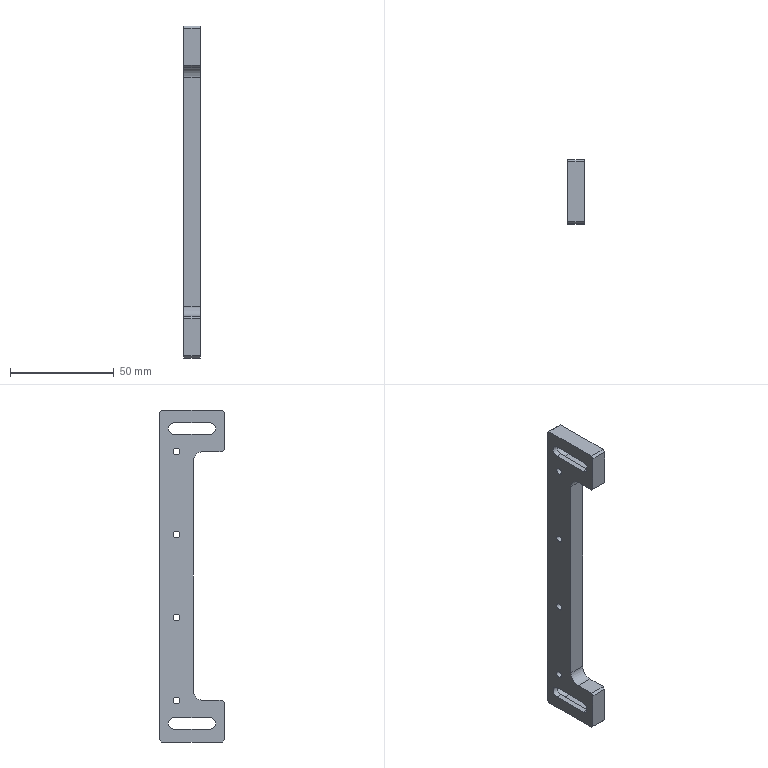Part | SolidWorks | features BaseBody 1 | 1 solid | 44 faces | box 8 x 31 x 160 mm | volume 21339 mm3 | plane 26 | cylinder 18 | commonest cylinder face diameters 3.3 x8 5.5 x4 11 x4 10 x2
STEP:
#1=CARTESIAN_POINT('',(-732.66,-691.086,-336.969));
#2=VERTEX_POINT('',#1);
#3=CARTESIAN_POINT('',(-732.66,-691.086,-333.669));
#4=VERTEX_POINT('',#3);
#5=CARTESIAN_POINT('',(-732.66,-691.086,-335.319));
#6=DIRECTION('',(-1.,0.,0.));
#7=DIRECTION('',(0.,0.,-1.));
#8=AXIS2_PLACEMENT_3D('',#5,#6,#7);
#9=CIRCLE('',#8,1.65);
#10=EDGE_CURVE('',#2,#4,#9,.T.);
#11=ORIENTED_EDGE('',*,*,#10,.T.);
#12=CARTESIAN_POINT('',(-724.66,-691.086,-333.669));
#13=VERTEX_POINT('',#12);
#14=CARTESIAN_POINT('',(-724.66,-691.086,-333.669));
#15=DIRECTION('',(1.,0.,0.));
#16=VECTOR('',#15,1000.);
#17=LINE('',#14,#16);
#18=EDGE_CURVE('',#4,#13,#17,.T.);
#19=ORIENTED_EDGE('',*,*,#18,.T.);
#20=CARTESIAN_POINT('',(-724.66,-691.086,-336.969));
#21=VERTEX_POINT('',#20);
#22=CARTESIAN_POINT('',(-724.66,-691.086,-335.319));
#23=DIRECTION('',(-1.,0.,0.));
#24=DIRECTION('',(0.,0.,-1.));
#25=AXIS2_PLACEMENT_3D('',#22,#23,#24);
#26=CIRCLE('',#25,1.65);
#27=EDGE_CURVE('',#21,#13,#26,.T.);
#28=ORIENTED_EDGE('',*,*,#27,.F.);
#29=CARTESIAN_POINT('',(-724.66,-691.086,-336.969));
#30=DIRECTION('',(1.,0.,0.));
#31=VECTOR('',#30,1000.);
#32=LINE('',#29,#31);
#33=EDGE_CURVE('',#2,#21,#32,.T.);
#34=ORIENTED_EDGE('',*,*,#33,.F.);
#35=EDGE_LOOP('',(#11,#19,#28,#34));
#36=FACE_OUTER_BOUND('',#35,.T.);
#37=CARTESIAN_POINT('',(-724.66,-691.086,-335.319));
#38=DIRECTION('',(1.,0.,0.));
#39=DIRECTION('',(0.,0.,-1.));
#40=AXIS2_PLACEMENT_3D('',#37,#38,#39);
#41=CYLINDRICAL_SURFACE('',#40,1.65);
#42=ADVANCED_FACE('',(#36),#41,.F.);
#43=CARTESIAN_POINT('',(-732.66,-691.086,-376.969));
#44=VERTEX_POINT('',#43);
#45=CARTESIAN_POINT('',(-732.66,-691.086,-373.669));
#46=VERTEX_POINT('',#45);
#47=CARTESIAN_POINT('',(-732.66,-691.086,-375.319));
#48=DIRECTION('',(-1.,0.,0.));
#49=DIRECTION('',(0.,0.,-1.));
#50=AXIS2_PLACEMENT_3D('',#47,#48,#49);
#51=CIRCLE('',#50,1.65);
#52=EDGE_CURVE('',#44,#46,#51,.T.);
#53=ORIENTED_EDGE('',*,*,#52,.T.);
#54=CARTESIAN_POINT('',(-724.66,-691.086,-373.669));
#55=VERTEX_POINT('',#54);
#56=CARTESIAN_POINT('',(-724.66,-691.086,-373.669));
#57=DIRECTION('',(1.,0.,0.));
#58=VECTOR('',#57,1000.);
#59=LINE('',#56,#58);
#60=EDGE_CURVE('',#46,#55,#59,.T.);
#61=ORIENTED_EDGE('',*,*,#60,.T.);
#62=CARTESIAN_POINT('',(-724.66,-691.086,-376.969));
#63=VERTEX_POINT('',#62);
#64=CARTESIAN_POINT('',(-724.66,-691.086,-375.319));
#65=DIRECTION('',(-1.,0.,0.));
#66=DIRECTION('',(0.,0.,-1.));
#67=AXIS2_PLACEMENT_3D('',#64,#65,#66);
#68=CIRCLE('',#67,1.65);
#69=EDGE_CURVE('',#63,#55,#68,.T.);
#70=ORIENTED_EDGE('',*,*,#69,.F.);
#71=CARTESIAN_POINT('',(-724.66,-691.086,-376.969));
#72=DIRECTION('',(1.,0.,0.));
#73=VECTOR('',#72,1000.);
#74=LINE('',#71,#73);
#75=EDGE_CURVE('',#44,#63,#74,.T.);
#76=ORIENTED_EDGE('',*,*,#75,.F.);
#77=EDGE_LOOP('',(#53,#61,#70,#76));
#78=FACE_OUTER_BOUND('',#77,.T.);
#79=CARTESIAN_POINT('',(-724.66,-691.086,-375.319));
#80=DIRECTION('',(1.,0.,0.));
#81=DIRECTION('',(0.,0.,-1.));
#82=AXIS2_PLACEMENT_3D('',#79,#80,#81);
#83=CYLINDRICAL_SURFACE('',#82,1.65);
#84=ADVANCED_FACE('',(#78),#83,.F.);
#85=CARTESIAN_POINT('',(-732.66,-691.086,-416.969));
#86=VERTEX_POINT('',#85);
#87=CARTESIAN_POINT('',(-732.66,-691.086,-413.669));
#88=VERTEX_POINT('',#87);
#89=CARTESIAN_POINT('',(-732.66,-691.086,-415.319));
#90=DIRECTION('',(-1.,0.,0.));
#91=DIRECTION('',(0.,0.,-1.));
#92=AXIS2_PLACEMENT_3D('',#89,#90,#91);
#93=CIRCLE('',#92,1.65);
#94=EDGE_CURVE('',#86,#88,#93,.T.);
#95=ORIENTED_EDGE('',*,*,#94,.T.);
#96=CARTESIAN_POINT('',(-724.66,-691.086,-413.669));
#97=VERTEX_POINT('',#96);
#98=CARTESIAN_POINT('',(-724.66,-691.086,-413.669));
#99=DIRECTION('',(1.,0.,0.));
#100=VECTOR('',#99,1000.);
#101=LINE('',#98,#100);
#102=EDGE_CURVE('',#88,#97,#101,.T.);
#103=ORIENTED_EDGE('',*,*,#102,.T.);
#104=CARTESIAN_POINT('',(-724.66,-691.086,-416.969));
#105=VERTEX_POINT('',#104);
#106=CARTESIAN_POINT('',(-724.66,-691.086,-415.319));
#107=DIRECTION('',(-1.,0.,0.));
#108=DIRECTION('',(0.,0.,-1.));
#109=AXIS2_PLACEMENT_3D('',#106,#107,#108);
#110=CIRCLE('',#109,1.65);
#111=EDGE_CURVE('',#105,#97,#110,.T.);
#112=ORIENTED_EDGE('',*,*,#111,.F.);
#113=CARTESIAN_POINT('',(-724.66,-691.086,-416.969));
#114=DIRECTION('',(1.,0.,0.));
#115=VECTOR('',#114,1000.);
#116=LINE('',#113,#115);
#117=EDGE_CURVE('',#86,#105,#116,.T.);
#118=ORIENTED_EDGE('',*,*,#117,.F.);
#119=EDGE_LOOP('',(#95,#103,#112,#118));
#120=FACE_OUTER_BOUND('',#119,.T.);
#121=CARTESIAN_POINT('',(-724.66,-691.086,-415.319));
#122=DIRECTION('',(1.,0.,0.));
#123=DIRECTION('',(0.,0.,-1.));
#124=AXIS2_PLACEMENT_3D('',#121,#122,#123);
#125=CYLINDRICAL_SURFACE('',#124,1.65);
#126=ADVANCED_FACE('',(#120),#125,.F.);
#127=CARTESIAN_POINT('',(-732.66,-691.086,-456.969));
#128=VERTEX_POINT('',#127);
#129=CARTESIAN_POINT('',(-732.66,-691.086,-453.669));
#130=VERTEX_POINT('',#129);
#131=CARTESIAN_POINT('',(-732.66,-691.086,-455.319));
#132=DIRECTION('',(-1.,0.,0.));
#133=DIRECTION('',(0.,0.,-1.));
#134=AXIS2_PLACEMENT_3D('',#131,#132,#133);
#135=CIRCLE('',#134,1.65);
#136=EDGE_CURVE('',#128,#130,#135,.T.);
#137=ORIENTED_EDGE('',*,*,#136,.T.);
#138=CARTESIAN_POINT('',(-724.66,-691.086,-453.669));
#139=VERTEX_POINT('',#138);
#140=CARTESIAN_POINT('',(-724.66,-691.086,-453.669));
#141=DIRECTION('',(1.,0.,0.));
#142=VECTOR('',#141,1000.);
#143=LINE('',#140,#142);
#144=EDGE_CURVE('',#130,#139,#143,.T.);
#145=ORIENTED_EDGE('',*,*,#144,.T.);
#146=CARTESIAN_POINT('',(-724.66,-691.086,-456.969));
#147=VERTEX_POINT('',#146);
#148=CARTESIAN_POINT('',(-724.66,-691.086,-455.319));
#149=DIRECTION('',(-1.,0.,0.));
#150=DIRECTION('',(0.,0.,-1.));
#151=AXIS2_PLACEMENT_3D('',#148,#149,#150);
#152=CIRCLE('',#151,1.65);
#153=EDGE_CURVE('',#147,#139,#152,.T.);
#154=ORIENTED_EDGE('',*,*,#153,.F.);
#155=CARTESIAN_POINT('',(-724.66,-691.086,-456.969));
#156=DIRECTION('',(1.,0.,0.));
#157=VECTOR('',#156,1000.);
#158=LINE('',#155,#157);
#159=EDGE_CURVE('',#128,#147,#158,.T.);
#160=ORIENTED_EDGE('',*,*,#159,.F.);
#161=EDGE_LOOP('',(#137,#145,#154,#160));
#162=FACE_OUTER_BOUND('',#161,.T.);
#163=CARTESIAN_POINT('',(-724.66,-691.086,-455.319));
#164=DIRECTION('',(1.,0.,0.));
#165=DIRECTION('',(0.,0.,-1.));
#166=AXIS2_PLACEMENT_3D('',#163,#164,#165);
#167=CYLINDRICAL_SURFACE('',#166,1.65);
#168=ADVANCED_FACE('',(#162),#167,.F.);
#169=ORIENTED_EDGE('',*,*,#10,.F.);
#170=CARTESIAN_POINT('',(-732.66,-691.086,-335.319));
#171=DIRECTION('',(-1.,0.,0.));
#172=DIRECTION('',(0.,0.,-1.));
#173=AXIS2_PLACEMENT_3D('',#170,#171,#172);
#174=CIRCLE('',#173,1.65);
#175=EDGE_CURVE('',#4,#2,#174,.T.);
#176=ORIENTED_EDGE('',*,*,#175,.F.);
#177=EDGE_LOOP('',(#169,#176));
#178=FACE_BOUND('',#177,.T.);
#179=ORIENTED_EDGE('',*,*,#52,.F.);
#180=CARTESIAN_POINT('',(-732.66,-691.086,-375.319));
#181=DIRECTION('',(-1.,0.,0.));
#182=DIRECTION('',(0.,0.,-1.));
#183=AXIS2_PLACEMENT_3D('',#180,#181,#182);
#184=CIRCLE('',#183,1.65);
#185=EDGE_CURVE('',#46,#44,#184,.T.);
#186=ORIENTED_EDGE('',*,*,#185,.F.);
#187=EDGE_LOOP('',(#179,#186));
#188=FACE_BOUND('',#187,.T.);
#189=ORIENTED_EDGE('',*,*,#94,.F.);
#190=CARTESIAN_POINT('',(-732.66,-691.086,-415.319));
#191=DIRECTION('',(-1.,0.,0.));
#192=DIRECTION('',(0.,0.,-1.));
#193=AXIS2_PLACEMENT_3D('',#190,#191,#192);
#194=CIRCLE('',#193,1.65);
#195=EDGE_CURVE('',#88,#86,#194,.T.);
#196=ORIENTED_EDGE('',*,*,#195,.F.);
#197=EDGE_LOOP('',(#189,#196));
#198=FACE_BOUND('',#197,.T.);
#199=ORIENTED_EDGE('',*,*,#136,.F.);
#200=CARTESIAN_POINT('',(-732.66,-691.086,-455.319));
#201=DIRECTION('',(-1.,0.,0.));
#202=DIRECTION('',(0.,0.,-1.));
#203=AXIS2_PLACEMENT_3D('',#200,#201,#202);
#204=CIRCLE('',#203,1.65);
#205=EDGE_CURVE('',#130,#128,#204,.T.);
#206=ORIENTED_EDGE('',*,*,#205,.F.);
#207=EDGE_LOOP('',(#199,#206));
#208=FACE_BOUND('',#207,.T.);
#209=CARTESIAN_POINT('',(-732.66,-707.336,-327.069));
#210=VERTEX_POINT('',#209);
#211=CARTESIAN_POINT('',(-732.66,-707.336,-321.569));
#212=VERTEX_POINT('',#211);
#213=CARTESIAN_POINT('',(-732.66,-707.336,-324.319));
#214=DIRECTION('',(-1.,0.,0.));
#215=DIRECTION('',(0.,0.,-1.));
#216=AXIS2_PLACEMENT_3D('',#213,#214,#215);
#217=CIRCLE('',#216,2.75);
#218=EDGE_CURVE('',#210,#212,#217,.T.);
#219=ORIENTED_EDGE('',*,*,#218,.F.);
#220=CARTESIAN_POINT('',(-732.66,-689.836,-327.069));
#221=VERTEX_POINT('',#220);
#222=CARTESIAN_POINT('',(-732.66,-691.086,-327.069));
#223=DIRECTION('',(0.,-1.,0.));
#224=VECTOR('',#223,1000.);
#225=LINE('',#222,#224);
#226=EDGE_CURVE('',#221,#210,#225,.T.);
#227=ORIENTED_EDGE('',*,*,#226,.F.);
#228=CARTESIAN_POINT('',(-732.66,-689.836,-321.569));
#229=VERTEX_POINT('',#228);
#230=CARTESIAN_POINT('',(-732.66,-689.836,-324.319));
#231=DIRECTION('',(-1.,0.,0.));
#232=DIRECTION('',(0.,0.,-1.));
#233=AXIS2_PLACEMENT_3D('',#230,#231,#232);
#234=CIRCLE('',#233,2.75);
#235=EDGE_CURVE('',#229,#221,#234,.T.);
#236=ORIENTED_EDGE('',*,*,#235,.F.);
#237=CARTESIAN_POINT('',(-732.66,-691.086,-321.569));
#238=DIRECTION('',(0.,1.,0.));
#239=VECTOR('',#238,1000.);
#240=LINE('',#237,#239);
#241=EDGE_CURVE('',#212,#229,#240,.T.);
#242=ORIENTED_EDGE('',*,*,#241,.F.);
#243=EDGE_LOOP('',(#219,#227,#236,#242));
#244=FACE_BOUND('',#243,.T.);
#245=CARTESIAN_POINT('',(-732.66,-707.336,-469.069));
#246=VERTEX_POINT('',#245);
#247=CARTESIAN_POINT('',(-732.66,-707.336,-463.569));
#248=VERTEX_POINT('',#247);
#249=CARTESIAN_POINT('',(-732.66,-707.336,-466.319));
#250=DIRECTION('',(-1.,0.,0.));
#251=DIRECTION('',(0.,0.,-1.));
#252=AXIS2_PLACEMENT_3D('',#249,#250,#251);
#253=CIRCLE('',#252,2.75);
#254=EDGE_CURVE('',#246,#248,#253,.T.);
#255=ORIENTED_EDGE('',*,*,#254,.F.);
#256=CARTESIAN_POINT('',(-732.66,-689.836,-469.069));
#257=VERTEX_POINT('',#256);
#258=CARTESIAN_POINT('',(-732.66,-691.086,-469.069));
#259=DIRECTION('',(0.,-1.,0.));
#260=VECTOR('',#259,1000.);
#261=LINE('',#258,#260);
#262=EDGE_CURVE('',#257,#246,#261,.T.);
#263=ORIENTED_EDGE('',*,*,#262,.F.);
#264=CARTESIAN_POINT('',(-732.66,-689.836,-463.569));
#265=VERTEX_POINT('',#264);
#266=CARTESIAN_POINT('',(-732.66,-689.836,-466.319));
#267=DIRECTION('',(-1.,0.,0.));
#268=DIRECTION('',(0.,0.,-1.));
#269=AXIS2_PLACEMENT_3D('',#266,#267,#268);
#270=CIRCLE('',#269,2.75);
#271=EDGE_CURVE('',#265,#257,#270,.T.);
#272=ORIENTED_EDGE('',*,*,#271,.F.);
#273=CARTESIAN_POINT('',(-732.66,-691.086,-463.569));
#274=DIRECTION('',(0.,1.,0.));
#275=VECTOR('',#274,1000.);
#276=LINE('',#273,#275);
#277=EDGE_CURVE('',#248,#265,#276,.T.);
#278=ORIENTED_EDGE('',*,*,#277,.F.);
#279=EDGE_LOOP('',(#255,#263,#272,#278));
#280=FACE_BOUND('',#279,.T.);
#281=CARTESIAN_POINT('',(-732.66,-713.086,-335.319));
#282=VERTEX_POINT('',#281);
#283=CARTESIAN_POINT('',(-732.66,-704.086,-335.319));
#284=VERTEX_POINT('',#283);
#285=CARTESIAN_POINT('',(-732.66,-691.086,-335.319));
#286=DIRECTION('',(0.,1.,0.));
#287=VECTOR('',#286,1000.);
#288=LINE('',#285,#287);
#289=EDGE_CURVE('',#282,#284,#288,.T.);
#290=ORIENTED_EDGE('',*,*,#289,.F.);
#291=CARTESIAN_POINT('',(-732.66,-714.086,-334.319));
#292=VERTEX_POINT('',#291);
#293=CARTESIAN_POINT('',(-732.66,-714.086,-334.319));
#294=DIRECTION('',(0.,-0.7071,0.7071));
#295=VECTOR('',#294,1000.);
#296=LINE('',#293,#295);
#297=EDGE_CURVE('',#282,#292,#296,.T.);
#298=ORIENTED_EDGE('',*,*,#297,.T.);
#299=CARTESIAN_POINT('',(-732.66,-714.086,-316.319));
#300=VERTEX_POINT('',#299);
#301=CARTESIAN_POINT('',(-732.66,-714.086,-395.319));
#302=DIRECTION('',(0.,0.,-1.));
#303=VECTOR('',#302,1000.);
#304=LINE('',#301,#303);
#305=EDGE_CURVE('',#300,#292,#304,.T.);
#306=ORIENTED_EDGE('',*,*,#305,.F.);
#307=CARTESIAN_POINT('',(-732.66,-713.086,-315.319));
#308=VERTEX_POINT('',#307);
#309=CARTESIAN_POINT('',(-732.66,-713.086,-315.319));
#310=DIRECTION('',(0.,-0.7071,-0.7071));
#311=VECTOR('',#310,1000.);
#312=LINE('',#309,#311);
#313=EDGE_CURVE('',#308,#300,#312,.T.);
#314=ORIENTED_EDGE('',*,*,#313,.F.);
#315=CARTESIAN_POINT('',(-732.66,-684.086,-315.319));
#316=VERTEX_POINT('',#315);
#317=CARTESIAN_POINT('',(-732.66,-691.086,-315.319));
#318=DIRECTION('',(0.,-1.,0.));
#319=VECTOR('',#318,1000.);
#320=LINE('',#317,#319);
#321=EDGE_CURVE('',#316,#308,#320,.T.);
#322=ORIENTED_EDGE('',*,*,#321,.F.);
#323=CARTESIAN_POINT('',(-732.66,-683.086,-316.319));
#324=VERTEX_POINT('',#323);
#325=CARTESIAN_POINT('',(-732.66,-684.086,-315.319));
#326=DIRECTION('',(0.,0.7071,-0.7071));
#327=VECTOR('',#326,1000.);
#328=LINE('',#325,#327);
#329=EDGE_CURVE('',#316,#324,#328,.T.);
#330=ORIENTED_EDGE('',*,*,#329,.T.);
#331=CARTESIAN_POINT('',(-732.66,-683.086,-474.319));
#332=VERTEX_POINT('',#331);
#333=CARTESIAN_POINT('',(-732.66,-683.086,-395.319));
#334=DIRECTION('',(0.,0.,1.));
#335=VECTOR('',#334,1000.);
#336=LINE('',#333,#335);
#337=EDGE_CURVE('',#332,#324,#336,.T.);
#338=ORIENTED_EDGE('',*,*,#337,.F.);
#339=CARTESIAN_POINT('',(-732.66,-684.086,-475.319));
#340=VERTEX_POINT('',#339);
#341=CARTESIAN_POINT('',(-732.66,-683.086,-474.319));
#342=DIRECTION('',(0.,-0.7071,-0.7071));
#343=VECTOR('',#342,1000.);
#344=LINE('',#341,#343);
#345=EDGE_CURVE('',#332,#340,#344,.T.);
#346=ORIENTED_EDGE('',*,*,#345,.T.);
#347=CARTESIAN_POINT('',(-732.66,-713.086,-475.319));
#348=VERTEX_POINT('',#347);
#349=CARTESIAN_POINT('',(-732.66,-691.086,-475.319));
#350=DIRECTION('',(0.,1.,0.));
#351=VECTOR('',#350,1000.);
#352=LINE('',#349,#351);
#353=EDGE_CURVE('',#348,#340,#352,.T.);
#354=ORIENTED_EDGE('',*,*,#353,.F.);
#355=CARTESIAN_POINT('',(-732.66,-714.086,-474.319));
#356=VERTEX_POINT('',#355);
#357=CARTESIAN_POINT('',(-732.66,-714.086,-474.319));
#358=DIRECTION('',(0.,0.7071,-0.7071));
#359=VECTOR('',#358,1000.);
#360=LINE('',#357,#359);
#361=EDGE_CURVE('',#356,#348,#360,.T.);
#362=ORIENTED_EDGE('',*,*,#361,.F.);
#363=CARTESIAN_POINT('',(-732.66,-714.086,-456.319));
#364=VERTEX_POINT('',#363);
#365=CARTESIAN_POINT('',(-732.66,-714.086,-395.319));
#366=DIRECTION('',(0.,0.,-1.));
#367=VECTOR('',#366,1000.);
#368=LINE('',#365,#367);
#369=EDGE_CURVE('',#364,#356,#368,.T.);
#370=ORIENTED_EDGE('',*,*,#369,.F.);
#371=CARTESIAN_POINT('',(-732.66,-713.086,-455.319));
#372=VERTEX_POINT('',#371);
#373=CARTESIAN_POINT('',(-732.66,-713.086,-455.319));
#374=DIRECTION('',(0.,0.7071,0.7071));
#375=VECTOR('',#374,1000.);
#376=LINE('',#373,#375);
#377=EDGE_CURVE('',#364,#372,#376,.T.);
#378=ORIENTED_EDGE('',*,*,#377,.T.);
#379=CARTESIAN_POINT('',(-732.66,-704.086,-455.319));
#380=VERTEX_POINT('',#379);
#381=CARTESIAN_POINT('',(-732.66,-691.086,-455.319));
#382=DIRECTION('',(0.,-1.,0.));
#383=VECTOR('',#382,1000.);
#384=LINE('',#381,#383);
#385=EDGE_CURVE('',#380,#372,#384,.T.);
#386=ORIENTED_EDGE('',*,*,#385,.F.);
#387=CARTESIAN_POINT('',(-732.66,-699.086,-450.319));
#388=VERTEX_POINT('',#387);
#389=CARTESIAN_POINT('',(-732.66,-704.086,-450.319));
#390=DIRECTION('',(-1.,0.,0.));
#391=DIRECTION('',(0.,0.,-1.));
#392=AXIS2_PLACEMENT_3D('',#389,#390,#391);
#393=CIRCLE('',#392,5.);
#394=EDGE_CURVE('',#388,#380,#393,.T.);
#395=ORIENTED_EDGE('',*,*,#394,.F.);
#396=CARTESIAN_POINT('',(-732.66,-699.086,-340.319));
#397=VERTEX_POINT('',#396);
#398=CARTESIAN_POINT('',(-732.66,-699.086,-395.319));
#399=DIRECTION('',(0.,0.,-1.));
#400=VECTOR('',#399,1000.);
#401=LINE('',#398,#400);
#402=EDGE_CURVE('',#397,#388,#401,.T.);
#403=ORIENTED_EDGE('',*,*,#402,.F.);
#404=CARTESIAN_POINT('',(-732.66,-704.086,-340.319));
#405=DIRECTION('',(-1.,0.,0.));
#406=DIRECTION('',(0.,0.,-1.));
#407=AXIS2_PLACEMENT_3D('',#404,#405,#406);
#408=CIRCLE('',#407,5.);
#409=EDGE_CURVE('',#284,#397,#408,.T.);
#410=ORIENTED_EDGE('',*,*,#409,.F.);
#411=EDGE_LOOP('',(#290,#298,#306,#314,#322,#330,#338,#346,#354,#362,#370,#378,#386,#395,#403,#410));
#412=FACE_OUTER_BOUND('',#411,.T.);
#413=CARTESIAN_POINT('',(-732.66,-691.086,-395.319));
#414=DIRECTION('',(1.,0.,0.));
#415=DIRECTION('',(0.,0.,-1.));
#416=AXIS2_PLACEMENT_3D('',#413,#414,#415);
#417=PLANE('',#416);
#418=ADVANCED_FACE('',(#178,#188,#198,#208,#244,#280,#412),#417,.F.);
#419=ORIENTED_EDGE('',*,*,#18,.F.);
#420=ORIENTED_EDGE('',*,*,#175,.T.);
#421=ORIENTED_EDGE('',*,*,#33,.T.);
#422=CARTESIAN_POINT('',(-724.66,-691.086,-335.319));
#423=DIRECTION('',(-1.,0.,0.));
#424=DIRECTION('',(0.,0.,-1.));
#425=AXIS2_PLACEMENT_3D('',#422,#423,#424);
#426=CIRCLE('',#425,1.65);
#427=EDGE_CURVE('',#13,#21,#426,.T.);
#428=ORIENTED_EDGE('',*,*,#427,.F.);
#429=EDGE_LOOP('',(#419,#420,#421,#428));
#430=FACE_OUTER_BOUND('',#429,.T.);
#431=CARTESIAN_POINT('',(-724.66,-691.086,-335.319));
#432=DIRECTION('',(1.,0.,0.));
#433=DIRECTION('',(0.,0.,-1.));
#434=AXIS2_PLACEMENT_3D('',#431,#432,#433);
#435=CYLINDRICAL_SURFACE('',#434,1.65);
#436=ADVANCED_FACE('',(#430),#435,.F.);
#437=ORIENTED_EDGE('',*,*,#60,.F.);
#438=ORIENTED_EDGE('',*,*,#185,.T.);
#439=ORIENTED_EDGE('',*,*,#75,.T.);
#440=CARTESIAN_POINT('',(-724.66,-691.086,-375.319));
#441=DIRECTION('',(-1.,0.,0.));
#442=DIRECTION('',(0.,0.,-1.));
#443=AXIS2_PLACEMENT_3D('',#440,#441,#442);
#444=CIRCLE('',#443,1.65);
#445=EDGE_CURVE('',#55,#63,#444,.T.);
#446=ORIENTED_EDGE('',*,*,#445,.F.);
#447=EDGE_LOOP('',(#437,#438,#439,#446));
#448=FACE_OUTER_BOUND('',#447,.T.);
#449=CARTESIAN_POINT('',(-724.66,-691.086,-375.319));
#450=DIRECTION('',(1.,0.,0.));
#451=DIRECTION('',(0.,0.,-1.));
#452=AXIS2_PLACEMENT_3D('',#449,#450,#451);
#453=CYLINDRICAL_SURFACE('',#452,1.65);
#454=ADVANCED_FACE('',(#448),#453,.F.);
#455=ORIENTED_EDGE('',*,*,#102,.F.);
#456=ORIENTED_EDGE('',*,*,#195,.T.);
#457=ORIENTED_EDGE('',*,*,#117,.T.);
#458=CARTESIAN_POINT('',(-724.66,-691.086,-415.319));
#459=DIRECTION('',(-1.,0.,0.));
#460=DIRECTION('',(0.,0.,-1.));
#461=AXIS2_PLACEMENT_3D('',#458,#459,#460);
#462=CIRCLE('',#461,1.65);
#463=EDGE_CURVE('',#97,#105,#462,.T.);
#464=ORIENTED_EDGE('',*,*,#463,.F.);
#465=EDGE_LOOP('',(#455,#456,#457,#464));
#466=FACE_OUTER_BOUND('',#465,.T.);
#467=CARTESIAN_POINT('',(-724.66,-691.086,-415.319));
#468=DIRECTION('',(1.,0.,0.));
#469=DIRECTION('',(0.,0.,-1.));
#470=AXIS2_PLACEMENT_3D('',#467,#468,#469);
#471=CYLINDRICAL_SURFACE('',#470,1.65);
#472=ADVANCED_FACE('',(#466),#471,.F.);
#473=ORIENTED_EDGE('',*,*,#144,.F.);
#474=ORIENTED_EDGE('',*,*,#205,.T.);
#475=ORIENTED_EDGE('',*,*,#159,.T.);
#476=CARTESIAN_POINT('',(-724.66,-691.086,-455.319));
#477=DIRECTION('',(-1.,0.,0.));
#478=DIRECTION('',(0.,0.,-1.));
#479=AXIS2_PLACEMENT_3D('',#476,#477,#478);
#480=CIRCLE('',#479,1.65);
#481=EDGE_CURVE('',#139,#147,#480,.T.);
#482=ORIENTED_EDGE('',*,*,#481,.F.);
#483=EDGE_LOOP('',(#473,#474,#475,#482));
#484=FACE_OUTER_BOUND('',#483,.T.);
#485=CARTESIAN_POINT('',(-724.66,-691.086,-455.319));
#486=DIRECTION('',(1.,0.,0.));
#487=DIRECTION('',(0.,0.,-1.));
#488=AXIS2_PLACEMENT_3D('',#485,#486,#487);
#489=CYLINDRICAL_SURFACE('',#488,1.65);
#490=ADVANCED_FACE('',(#484),#489,.F.);
#491=CARTESIAN_POINT('',(-730.06,-707.336,-321.569));
#492=VERTEX_POINT('',#491);
#493=CARTESIAN_POINT('',(-724.66,-707.336,-321.569));
#494=DIRECTION('',(1.,0.,0.));
#495=VECTOR('',#494,1000.);
#496=LINE('',#493,#495);
#497=EDGE_CURVE('',#212,#492,#496,.T.);
#498=ORIENTED_EDGE('',*,*,#497,.F.);
#499=ORIENTED_EDGE('',*,*,#241,.T.);
#500=CARTESIAN_POINT('',(-730.06,-689.836,-321.569));
#501=VERTEX_POINT('',#500);
#502=CARTESIAN_POINT('',(-724.66,-689.836,-321.569));
#503=DIRECTION('',(-1.,0.,0.));
#504=VECTOR('',#503,1000.);
#505=LINE('',#502,#504);
#506=EDGE_CURVE('',#501,#229,#505,.T.);
#507=ORIENTED_EDGE('',*,*,#506,.F.);
#508=CARTESIAN_POINT('',(-730.06,-707.336,-321.569));
#509=DIRECTION('',(0.,1.,0.));
#510=VECTOR('',#509,1000.);
#511=LINE('',#508,#510);
#512=EDGE_CURVE('',#492,#501,#511,.T.);
#513=ORIENTED_EDGE('',*,*,#512,.F.);
#514=EDGE_LOOP('',(#498,#499,#507,#513));
#515=FACE_OUTER_BOUND('',#514,.T.);
#516=CARTESIAN_POINT('',(-724.66,-707.336,-321.569));
#517=DIRECTION('',(0.,0.,1.));
#518=DIRECTION('',(1.,0.,0.));
#519=AXIS2_PLACEMENT_3D('',#516,#517,#518);
#520=PLANE('',#519);
#521=ADVANCED_FACE('',(#515),#520,.F.);
#522=CARTESIAN_POINT('',(-730.06,-707.336,-327.069));
#523=VERTEX_POINT('',#522);
#524=CARTESIAN_POINT('',(-724.66,-707.336,-327.069));
#525=DIRECTION('',(1.,0.,0.));
#526=VECTOR('',#525,1000.);
#527=LINE('',#524,#526);
#528=EDGE_CURVE('',#210,#523,#527,.T.);
#529=ORIENTED_EDGE('',*,*,#528,.F.);
#530=ORIENTED_EDGE('',*,*,#218,.T.);
#531=ORIENTED_EDGE('',*,*,#497,.T.);
#532=CARTESIAN_POINT('',(-730.06,-707.336,-324.319));
#533=DIRECTION('',(-1.,0.,0.));
#534=DIRECTION('',(0.,0.,-1.));
#535=AXIS2_PLACEMENT_3D('',#532,#533,#534);
#536=CIRCLE('',#535,2.75);
#537=EDGE_CURVE('',#523,#492,#536,.T.);
#538=ORIENTED_EDGE('',*,*,#537,.F.);
#539=EDGE_LOOP('',(#529,#530,#531,#538));
#540=FACE_OUTER_BOUND('',#539,.T.);
#541=CARTESIAN_POINT('',(-724.66,-707.336,-324.319));
#542=DIRECTION('',(1.,0.,0.));
#543=DIRECTION('',(0.,0.,-1.));
#544=AXIS2_PLACEMENT_3D('',#541,#542,#543);
#545=CYLINDRICAL_SURFACE('',#544,2.75);
#546=ADVANCED_FACE('',(#540),#545,.F.);
#547=CARTESIAN_POINT('',(-730.06,-689.836,-327.069));
#548=VERTEX_POINT('',#547);
#549=CARTESIAN_POINT('',(-732.66,-689.836,-327.069));
#550=DIRECTION('',(1.,0.,0.));
#551=VECTOR('',#550,1000.);
#552=LINE('',#549,#551);
#553=EDGE_CURVE('',#221,#548,#552,.T.);
#554=ORIENTED_EDGE('',*,*,#553,.F.);
#555=ORIENTED_EDGE('',*,*,#226,.T.);
#556=ORIENTED_EDGE('',*,*,#528,.T.);
#557=CARTESIAN_POINT('',(-730.06,-707.336,-327.069));
#558=DIRECTION('',(0.,-1.,0.));
#559=VECTOR('',#558,1000.);
#560=LINE('',#557,#559);
#561=EDGE_CURVE('',#548,#523,#560,.T.);
#562=ORIENTED_EDGE('',*,*,#561,.F.);
#563=EDGE_LOOP('',(#554,#555,#556,#562));
#564=FACE_OUTER_BOUND('',#563,.T.);
#565=CARTESIAN_POINT('',(-732.66,-707.336,-327.069));
#566=DIRECTION('',(0.,0.,-1.));
#567=DIRECTION('',(0.,1.,0.));
#568=AXIS2_PLACEMENT_3D('',#565,#566,#567);
#569=PLANE('',#568);
#570=ADVANCED_FACE('',(#564),#569,.F.);
#571=ORIENTED_EDGE('',*,*,#506,.T.);
#572=ORIENTED_EDGE('',*,*,#235,.T.);
#573=ORIENTED_EDGE('',*,*,#553,.T.);
#574=CARTESIAN_POINT('',(-730.06,-689.836,-324.319));
#575=DIRECTION('',(-1.,0.,0.));
#576=DIRECTION('',(0.,0.,-1.));
#577=AXIS2_PLACEMENT_3D('',#574,#575,#576);
#578=CIRCLE('',#577,2.75);
#579=EDGE_CURVE('',#501,#548,#578,.T.);
#580=ORIENTED_EDGE('',*,*,#579,.F.);
#581=EDGE_LOOP('',(#571,#572,#573,#580));
#582=FACE_OUTER_BOUND('',#581,.T.);
#583=CARTESIAN_POINT('',(-724.66,-689.836,-324.319));
#584=DIRECTION('',(1.,0.,0.));
#585=DIRECTION('',(0.,0.,-1.));
#586=AXIS2_PLACEMENT_3D('',#583,#584,#585);
#587=CYLINDRICAL_SURFACE('',#586,2.75);
#588=ADVANCED_FACE('',(#582),#587,.F.);
#589=CARTESIAN_POINT('',(-730.06,-707.336,-463.569));
#590=VERTEX_POINT('',#589);
#591=CARTESIAN_POINT('',(-724.66,-707.336,-463.569));
#592=DIRECTION('',(1.,0.,0.));
#593=VECTOR('',#592,1000.);
#594=LINE('',#591,#593);
#595=EDGE_CURVE('',#248,#590,#594,.T.);
#596=ORIENTED_EDGE('',*,*,#595,.F.);
#597=ORIENTED_EDGE('',*,*,#277,.T.);
#598=CARTESIAN_POINT('',(-730.06,-689.836,-463.569));
#599=VERTEX_POINT('',#598);
#600=CARTESIAN_POINT('',(-724.66,-689.836,-463.569));
#601=DIRECTION('',(-1.,0.,0.));
#602=VECTOR('',#601,1000.);
#603=LINE('',#600,#602);
#604=EDGE_CURVE('',#599,#265,#603,.T.);
#605=ORIENTED_EDGE('',*,*,#604,.F.);
#606=CARTESIAN_POINT('',(-730.06,-707.336,-463.569));
#607=DIRECTION('',(0.,1.,0.));
#608=VECTOR('',#607,1000.);
#609=LINE('',#606,#608);
#610=EDGE_CURVE('',#590,#599,#609,.T.);
#611=ORIENTED_EDGE('',*,*,#610,.F.);
#612=EDGE_LOOP('',(#596,#597,#605,#611));
#613=FACE_OUTER_BOUND('',#612,.T.);
#614=CARTESIAN_POINT('',(-724.66,-707.336,-463.569));
#615=DIRECTION('',(0.,0.,1.));
#616=DIRECTION('',(1.,0.,0.));
#617=AXIS2_PLACEMENT_3D('',#614,#615,#616);
#618=PLANE('',#617);
#619=ADVANCED_FACE('',(#613),#618,.F.);
#620=CARTESIAN_POINT('',(-730.06,-707.336,-469.069));
#621=VERTEX_POINT('',#620);
#622=CARTESIAN_POINT('',(-724.66,-707.336,-469.069));
#623=DIRECTION('',(1.,0.,0.));
#624=VECTOR('',#623,1000.);
#625=LINE('',#622,#624);
#626=EDGE_CURVE('',#246,#621,#625,.T.);
#627=ORIENTED_EDGE('',*,*,#626,.F.);
#628=ORIENTED_EDGE('',*,*,#254,.T.);
#629=ORIENTED_EDGE('',*,*,#595,.T.);
#630=CARTESIAN_POINT('',(-730.06,-707.336,-466.319));
#631=DIRECTION('',(-1.,0.,0.));
#632=DIRECTION('',(0.,0.,-1.));
#633=AXIS2_PLACEMENT_3D('',#630,#631,#632);
#634=CIRCLE('',#633,2.75);
#635=EDGE_CURVE('',#621,#590,#634,.T.);
#636=ORIENTED_EDGE('',*,*,#635,.F.);
#637=EDGE_LOOP('',(#627,#628,#629,#636));
#638=FACE_OUTER_BOUND('',#637,.T.);
#639=CARTESIAN_POINT('',(-724.66,-707.336,-466.319));
#640=DIRECTION('',(1.,0.,0.));
#641=DIRECTION('',(0.,0.,-1.));
#642=AXIS2_PLACEMENT_3D('',#639,#640,#641);
#643=CYLINDRICAL_SURFACE('',#642,2.75);
#644=ADVANCED_FACE('',(#638),#643,.F.);
#645=CARTESIAN_POINT('',(-730.06,-689.836,-469.069));
#646=VERTEX_POINT('',#645);
#647=CARTESIAN_POINT('',(-732.66,-689.836,-469.069));
#648=DIRECTION('',(1.,0.,0.));
#649=VECTOR('',#648,1000.);
#650=LINE('',#647,#649);
#651=EDGE_CURVE('',#257,#646,#650,.T.);
#652=ORIENTED_EDGE('',*,*,#651,.F.);
#653=ORIENTED_EDGE('',*,*,#262,.T.);
#654=ORIENTED_EDGE('',*,*,#626,.T.);
#655=CARTESIAN_POINT('',(-730.06,-707.336,-469.069));
#656=DIRECTION('',(0.,-1.,0.));
#657=VECTOR('',#656,1000.);
#658=LINE('',#655,#657);
#659=EDGE_CURVE('',#646,#621,#658,.T.);
#660=ORIENTED_EDGE('',*,*,#659,.F.);
#661=EDGE_LOOP('',(#652,#653,#654,#660));
#662=FACE_OUTER_BOUND('',#661,.T.);
#663=CARTESIAN_POINT('',(-732.66,-707.336,-469.069));
#664=DIRECTION('',(0.,0.,-1.));
#665=DIRECTION('',(0.,1.,0.));
#666=AXIS2_PLACEMENT_3D('',#663,#664,#665);
#667=PLANE('',#666);
#668=ADVANCED_FACE('',(#662),#667,.F.);
#669=ORIENTED_EDGE('',*,*,#604,.T.);
#670=ORIENTED_EDGE('',*,*,#271,.T.);
#671=ORIENTED_EDGE('',*,*,#651,.T.);
#672=CARTESIAN_POINT('',(-730.06,-689.836,-466.319));
#673=DIRECTION('',(-1.,0.,0.));
#674=DIRECTION('',(0.,0.,-1.));
#675=AXIS2_PLACEMENT_3D('',#672,#673,#674);
#676=CIRCLE('',#675,2.75);
#677=EDGE_CURVE('',#599,#646,#676,.T.);
#678=ORIENTED_EDGE('',*,*,#677,.F.);
#679=EDGE_LOOP('',(#669,#670,#671,#678));
#680=FACE_OUTER_BOUND('',#679,.T.);
#681=CARTESIAN_POINT('',(-724.66,-689.836,-466.319));
#682=DIRECTION('',(1.,0.,0.));
#683=DIRECTION('',(0.,0.,-1.));
#684=AXIS2_PLACEMENT_3D('',#681,#682,#683);
#685=CYLINDRICAL_SURFACE('',#684,2.75);
#686=ADVANCED_FACE('',(#680),#685,.F.);
#687=CARTESIAN_POINT('',(-724.66,-704.086,-335.319));
#688=VERTEX_POINT('',#687);
#689=CARTESIAN_POINT('',(-724.66,-699.086,-340.319));
#690=VERTEX_POINT('',#689);
#691=CARTESIAN_POINT('',(-724.66,-704.086,-340.319));
#692=DIRECTION('',(-1.,0.,0.));
#693=DIRECTION('',(0.,0.,-1.));
#694=AXIS2_PLACEMENT_3D('',#691,#692,#693);
#695=CIRCLE('',#694,5.);
#696=EDGE_CURVE('',#688,#690,#695,.T.);
#697=ORIENTED_EDGE('',*,*,#696,.F.);
#698=CARTESIAN_POINT('',(-732.66,-704.086,-335.319));
#699=DIRECTION('',(1.,0.,0.));
#700=VECTOR('',#699,1000.);
#701=LINE('',#698,#700);
#702=EDGE_CURVE('',#284,#688,#701,.T.);
#703=ORIENTED_EDGE('',*,*,#702,.F.);
#704=ORIENTED_EDGE('',*,*,#409,.T.);
#705=CARTESIAN_POINT('',(-732.66,-699.086,-340.319));
#706=DIRECTION('',(-1.,0.,0.));
#707=VECTOR('',#706,1000.);
#708=LINE('',#705,#707);
#709=EDGE_CURVE('',#690,#397,#708,.T.);
#710=ORIENTED_EDGE('',*,*,#709,.F.);
#711=EDGE_LOOP('',(#697,#703,#704,#710));
#712=FACE_OUTER_BOUND('',#711,.T.);
#713=CARTESIAN_POINT('',(-732.66,-704.086,-340.319));
#714=DIRECTION('',(1.,0.,0.));
#715=DIRECTION('',(0.,0.,-1.));
#716=AXIS2_PLACEMENT_3D('',#713,#714,#715);
#717=CYLINDRICAL_SURFACE('',#716,5.);
#718=ADVANCED_FACE('',(#712),#717,.F.);
#719=CARTESIAN_POINT('',(-724.66,-713.086,-335.319));
#720=VERTEX_POINT('',#719);
#721=CARTESIAN_POINT('',(-724.66,-699.086,-335.319));
#722=DIRECTION('',(0.,-1.,0.));
#723=VECTOR('',#722,1000.);
#724=LINE('',#721,#723);
#725=EDGE_CURVE('',#688,#720,#724,.T.);
#726=ORIENTED_EDGE('',*,*,#725,.T.);
#727=CARTESIAN_POINT('',(-732.66,-713.086,-335.319));
#728=DIRECTION('',(-1.,0.,0.));
#729=VECTOR('',#728,1000.);
#730=LINE('',#727,#729);
#731=EDGE_CURVE('',#720,#282,#730,.T.);
#732=ORIENTED_EDGE('',*,*,#731,.T.);
#733=ORIENTED_EDGE('',*,*,#289,.T.);
#734=ORIENTED_EDGE('',*,*,#702,.T.);
#735=EDGE_LOOP('',(#726,#732,#733,#734));
#736=FACE_OUTER_BOUND('',#735,.T.);
#737=CARTESIAN_POINT('',(-732.66,-699.086,-335.319));
#738=DIRECTION('',(0.,0.,-1.));
#739=DIRECTION('',(-1.,0.,0.));
#740=AXIS2_PLACEMENT_3D('',#737,#738,#739);
#741=PLANE('',#740);
#742=ADVANCED_FACE('',(#736),#741,.T.);
#743=ORIENTED_EDGE('',*,*,#305,.T.);
#744=CARTESIAN_POINT('',(-724.66,-714.086,-334.319));
#745=VERTEX_POINT('',#744);
#746=CARTESIAN_POINT('',(-732.66,-714.086,-334.319));
#747=DIRECTION('',(1.,0.,0.));
#748=VECTOR('',#747,1000.);
#749=LINE('',#746,#748);
#750=EDGE_CURVE('',#292,#745,#749,.T.);
#751=ORIENTED_EDGE('',*,*,#750,.T.);
#752=CARTESIAN_POINT('',(-724.66,-714.086,-316.319));
#753=VERTEX_POINT('',#752);
#754=CARTESIAN_POINT('',(-724.66,-714.086,-315.319));
#755=DIRECTION('',(0.,0.,1.));
#756=VECTOR('',#755,1000.);
#757=LINE('',#754,#756);
#758=EDGE_CURVE('',#745,#753,#757,.T.);
#759=ORIENTED_EDGE('',*,*,#758,.T.);
#760=CARTESIAN_POINT('',(-732.66,-714.086,-316.319));
#761=DIRECTION('',(-1.,0.,0.));
#762=VECTOR('',#761,1000.);
#763=LINE('',#760,#762);
#764=EDGE_CURVE('',#753,#300,#763,.T.);
#765=ORIENTED_EDGE('',*,*,#764,.T.);
#766=EDGE_LOOP('',(#743,#751,#759,#765));
#767=FACE_OUTER_BOUND('',#766,.T.);
#768=CARTESIAN_POINT('',(-732.66,-714.086,-315.319));
#769=DIRECTION('',(0.,-1.,0.));
#770=DIRECTION('',(0.,0.,-1.));
#771=AXIS2_PLACEMENT_3D('',#768,#769,#770);
#772=PLANE('',#771);
#773=ADVANCED_FACE('',(#767),#772,.T.);
#774=CARTESIAN_POINT('',(-724.66,-684.086,-315.319));
#775=VERTEX_POINT('',#774);
#776=CARTESIAN_POINT('',(-724.66,-713.086,-315.319));
#777=VERTEX_POINT('',#776);
#778=CARTESIAN_POINT('',(-724.66,-683.086,-315.319));
#779=DIRECTION('',(0.,-1.,0.));
#780=VECTOR('',#779,1000.);
#781=LINE('',#778,#780);
#782=EDGE_CURVE('',#775,#777,#781,.T.);
#783=ORIENTED_EDGE('',*,*,#782,.F.);
#784=CARTESIAN_POINT('',(-724.66,-684.086,-315.319));
#785=DIRECTION('',(1.,0.,0.));
#786=VECTOR('',#785,1000.);
#787=LINE('',#784,#786);
#788=EDGE_CURVE('',#316,#775,#787,.T.);
#789=ORIENTED_EDGE('',*,*,#788,.F.);
#790=ORIENTED_EDGE('',*,*,#321,.T.);
#791=CARTESIAN_POINT('',(-724.66,-713.086,-315.319));
#792=DIRECTION('',(-1.,0.,0.));
#793=VECTOR('',#792,1000.);
#794=LINE('',#791,#793);
#795=EDGE_CURVE('',#777,#308,#794,.T.);
#796=ORIENTED_EDGE('',*,*,#795,.F.);
#797=EDGE_LOOP('',(#783,#789,#790,#796));
#798=FACE_OUTER_BOUND('',#797,.T.);
#799=CARTESIAN_POINT('',(-724.66,-683.086,-315.319));
#800=DIRECTION('',(0.,0.,-1.));
#801=DIRECTION('',(-1.,0.,0.));
#802=AXIS2_PLACEMENT_3D('',#799,#800,#801);
#803=PLANE('',#802);
#804=ADVANCED_FACE('',(#798),#803,.F.);
#805=ORIENTED_EDGE('',*,*,#337,.T.);
#806=CARTESIAN_POINT('',(-724.66,-683.086,-316.319));
#807=VERTEX_POINT('',#806);
#808=CARTESIAN_POINT('',(-724.66,-683.086,-316.319));
#809=DIRECTION('',(-1.,0.,0.));
#810=VECTOR('',#809,1000.);
#811=LINE('',#808,#810);
#812=EDGE_CURVE('',#807,#324,#811,.T.);
#813=ORIENTED_EDGE('',*,*,#812,.F.);
#814=CARTESIAN_POINT('',(-724.66,-683.086,-474.319));
#815=VERTEX_POINT('',#814);
#816=CARTESIAN_POINT('',(-724.66,-683.086,-315.319));
#817=DIRECTION('',(0.,0.,1.));
#818=VECTOR('',#817,1000.);
#819=LINE('',#816,#818);
#820=EDGE_CURVE('',#815,#807,#819,.T.);
#821=ORIENTED_EDGE('',*,*,#820,.F.);
#822=CARTESIAN_POINT('',(-724.66,-683.086,-474.319));
#823=DIRECTION('',(1.,0.,0.));
#824=VECTOR('',#823,1000.);
#825=LINE('',#822,#824);
#826=EDGE_CURVE('',#332,#815,#825,.T.);
#827=ORIENTED_EDGE('',*,*,#826,.F.);
#828=EDGE_LOOP('',(#805,#813,#821,#827));
#829=FACE_OUTER_BOUND('',#828,.T.);
#830=CARTESIAN_POINT('',(-724.66,-683.086,-315.319));
#831=DIRECTION('',(0.,-1.,0.));
#832=DIRECTION('',(1.,0.,0.));
#833=AXIS2_PLACEMENT_3D('',#830,#831,#832);
#834=PLANE('',#833);
#835=ADVANCED_FACE('',(#829),#834,.F.);
#836=ORIENTED_EDGE('',*,*,#353,.T.);
#837=CARTESIAN_POINT('',(-724.66,-684.086,-475.319));
#838=VERTEX_POINT('',#837);
#839=CARTESIAN_POINT('',(-724.66,-684.086,-475.319));
#840=DIRECTION('',(-1.,0.,0.));
#841=VECTOR('',#840,1000.);
#842=LINE('',#839,#841);
#843=EDGE_CURVE('',#838,#340,#842,.T.);
#844=ORIENTED_EDGE('',*,*,#843,.F.);
#845=CARTESIAN_POINT('',(-724.66,-713.086,-475.319));
#846=VERTEX_POINT('',#845);
#847=CARTESIAN_POINT('',(-724.66,-683.086,-475.319));
#848=DIRECTION('',(0.,1.,0.));
#849=VECTOR('',#848,1000.);
#850=LINE('',#847,#849);
#851=EDGE_CURVE('',#846,#838,#850,.T.);
#852=ORIENTED_EDGE('',*,*,#851,.F.);
#853=CARTESIAN_POINT('',(-724.66,-713.086,-475.319));
#854=DIRECTION('',(1.,0.,0.));
#855=VECTOR('',#854,1000.);
#856=LINE('',#853,#855);
#857=EDGE_CURVE('',#348,#846,#856,.T.);
#858=ORIENTED_EDGE('',*,*,#857,.F.);
#859=EDGE_LOOP('',(#836,#844,#852,#858));
#860=FACE_OUTER_BOUND('',#859,.T.);
#861=CARTESIAN_POINT('',(-724.66,-683.086,-475.319));
#862=DIRECTION('',(0.,0.,1.));
#863=DIRECTION('',(1.,0.,0.));
#864=AXIS2_PLACEMENT_3D('',#861,#862,#863);
#865=PLANE('',#864);
#866=ADVANCED_FACE('',(#860),#865,.F.);
#867=CARTESIAN_POINT('',(-724.66,-714.086,-474.319));
#868=VERTEX_POINT('',#867);
#869=CARTESIAN_POINT('',(-724.66,-714.086,-456.319));
#870=VERTEX_POINT('',#869);
#871=CARTESIAN_POINT('',(-724.66,-714.086,-475.319));
#872=DIRECTION('',(0.,0.,1.));
#873=VECTOR('',#872,1000.);
#874=LINE('',#871,#873);
#875=EDGE_CURVE('',#868,#870,#874,.T.);
#876=ORIENTED_EDGE('',*,*,#875,.T.);
#877=CARTESIAN_POINT('',(-732.66,-714.086,-456.319));
#878=DIRECTION('',(-1.,0.,0.));
#879=VECTOR('',#878,1000.);
#880=LINE('',#877,#879);
#881=EDGE_CURVE('',#870,#364,#880,.T.);
#882=ORIENTED_EDGE('',*,*,#881,.T.);
#883=ORIENTED_EDGE('',*,*,#369,.T.);
#884=CARTESIAN_POINT('',(-732.66,-714.086,-474.319));
#885=DIRECTION('',(1.,0.,0.));
#886=VECTOR('',#885,1000.);
#887=LINE('',#884,#886);
#888=EDGE_CURVE('',#356,#868,#887,.T.);
#889=ORIENTED_EDGE('',*,*,#888,.T.);
#890=EDGE_LOOP('',(#876,#882,#883,#889));
#891=FACE_OUTER_BOUND('',#890,.T.);
#892=CARTESIAN_POINT('',(-732.66,-714.086,-475.319));
#893=DIRECTION('',(0.,-1.,0.));
#894=DIRECTION('',(0.,0.,-1.));
#895=AXIS2_PLACEMENT_3D('',#892,#893,#894);
#896=PLANE('',#895);
#897=ADVANCED_FACE('',(#891),#896,.T.);
#898=ORIENTED_EDGE('',*,*,#385,.T.);
#899=CARTESIAN_POINT('',(-724.66,-713.086,-455.319));
#900=VERTEX_POINT('',#899);
#901=CARTESIAN_POINT('',(-732.66,-713.086,-455.319));
#902=DIRECTION('',(1.,0.,0.));
#903=VECTOR('',#902,1000.);
#904=LINE('',#901,#903);
#905=EDGE_CURVE('',#372,#900,#904,.T.);
#906=ORIENTED_EDGE('',*,*,#905,.T.);
#907=CARTESIAN_POINT('',(-724.66,-704.086,-455.319));
#908=VERTEX_POINT('',#907);
#909=CARTESIAN_POINT('',(-724.66,-699.086,-455.319));
#910=DIRECTION('',(0.,1.,0.));
#911=VECTOR('',#910,1000.);
#912=LINE('',#909,#911);
#913=EDGE_CURVE('',#900,#908,#912,.T.);
#914=ORIENTED_EDGE('',*,*,#913,.T.);
#915=CARTESIAN_POINT('',(-732.66,-704.086,-455.319));
#916=DIRECTION('',(-1.,0.,0.));
#917=VECTOR('',#916,1000.);
#918=LINE('',#915,#917);
#919=EDGE_CURVE('',#908,#380,#918,.T.);
#920=ORIENTED_EDGE('',*,*,#919,.T.);
#921=EDGE_LOOP('',(#898,#906,#914,#920));
#922=FACE_OUTER_BOUND('',#921,.T.);
#923=CARTESIAN_POINT('',(-732.66,-699.086,-455.319));
#924=DIRECTION('',(0.,0.,1.));
#925=DIRECTION('',(1.,0.,0.));
#926=AXIS2_PLACEMENT_3D('',#923,#924,#925);
#927=PLANE('',#926);
#928=ADVANCED_FACE('',(#922),#927,.T.);
#929=CARTESIAN_POINT('',(-724.66,-699.086,-450.319));
#930=VERTEX_POINT('',#929);
#931=CARTESIAN_POINT('',(-724.66,-704.086,-450.319));
#932=DIRECTION('',(-1.,0.,0.));
#933=DIRECTION('',(0.,0.,-1.));
#934=AXIS2_PLACEMENT_3D('',#931,#932,#933);
#935=CIRCLE('',#934,5.);
#936=EDGE_CURVE('',#930,#908,#935,.T.);
#937=ORIENTED_EDGE('',*,*,#936,.F.);
#938=CARTESIAN_POINT('',(-724.66,-699.086,-450.319));
#939=DIRECTION('',(1.,0.,0.));
#940=VECTOR('',#939,1000.);
#941=LINE('',#938,#940);
#942=EDGE_CURVE('',#388,#930,#941,.T.);
#943=ORIENTED_EDGE('',*,*,#942,.F.);
#944=ORIENTED_EDGE('',*,*,#394,.T.);
#945=ORIENTED_EDGE('',*,*,#919,.F.);
#946=EDGE_LOOP('',(#937,#943,#944,#945));
#947=FACE_OUTER_BOUND('',#946,.T.);
#948=CARTESIAN_POINT('',(-724.66,-704.086,-450.319));
#949=DIRECTION('',(1.,0.,0.));
#950=DIRECTION('',(0.,0.,-1.));
#951=AXIS2_PLACEMENT_3D('',#948,#949,#950);
#952=CYLINDRICAL_SURFACE('',#951,5.);
#953=ADVANCED_FACE('',(#947),#952,.F.);
#954=CARTESIAN_POINT('',(-724.66,-699.086,-315.319));
#955=DIRECTION('',(0.,0.,-1.));
#956=VECTOR('',#955,1000.);
#957=LINE('',#954,#956);
#958=EDGE_CURVE('',#690,#930,#957,.T.);
#959=ORIENTED_EDGE('',*,*,#958,.F.);
#960=ORIENTED_EDGE('',*,*,#709,.T.);
#961=ORIENTED_EDGE('',*,*,#402,.T.);
#962=ORIENTED_EDGE('',*,*,#942,.T.);
#963=EDGE_LOOP('',(#959,#960,#961,#962));
#964=FACE_OUTER_BOUND('',#963,.T.);
#965=CARTESIAN_POINT('',(-724.66,-699.086,-315.319));
#966=DIRECTION('',(0.,1.,0.));
#967=DIRECTION('',(0.,0.,1.));
#968=AXIS2_PLACEMENT_3D('',#965,#966,#967);
#969=PLANE('',#968);
#970=ADVANCED_FACE('',(#964),#969,.F.);
#971=ORIENTED_EDGE('',*,*,#27,.T.);
#972=ORIENTED_EDGE('',*,*,#427,.T.);
#973=EDGE_LOOP('',(#971,#972));
#974=FACE_BOUND('',#973,.T.);
#975=ORIENTED_EDGE('',*,*,#69,.T.);
#976=ORIENTED_EDGE('',*,*,#445,.T.);
#977=EDGE_LOOP('',(#975,#976));
#978=FACE_BOUND('',#977,.T.);
#979=ORIENTED_EDGE('',*,*,#111,.T.);
#980=ORIENTED_EDGE('',*,*,#463,.T.);
#981=EDGE_LOOP('',(#979,#980));
#982=FACE_BOUND('',#981,.T.);
#983=ORIENTED_EDGE('',*,*,#153,.T.);
#984=ORIENTED_EDGE('',*,*,#481,.T.);
#985=EDGE_LOOP('',(#983,#984));
#986=FACE_BOUND('',#985,.T.);
#987=CARTESIAN_POINT('',(-724.66,-689.836,-318.819));
#988=VERTEX_POINT('',#987);
#989=CARTESIAN_POINT('',(-724.66,-689.836,-329.819));
#990=VERTEX_POINT('',#989);
#991=CARTESIAN_POINT('',(-724.66,-689.836,-324.319));
#992=DIRECTION('',(-1.,0.,0.));
#993=DIRECTION('',(0.,0.,-1.));
#994=AXIS2_PLACEMENT_3D('',#991,#992,#993);
#995=CIRCLE('',#994,5.5);
#996=EDGE_CURVE('',#988,#990,#995,.T.);
#997=ORIENTED_EDGE('',*,*,#996,.T.);
#998=CARTESIAN_POINT('',(-724.66,-707.336,-329.819));
#999=VERTEX_POINT('',#998);
#1000=CARTESIAN_POINT('',(-724.66,-691.086,-329.819));
#1001=DIRECTION('',(0.,-1.,0.));
#1002=VECTOR('',#1001,1000.);
#1003=LINE('',#1000,#1002);
#1004=EDGE_CURVE('',#990,#999,#1003,.T.);
#1005=ORIENTED_EDGE('',*,*,#1004,.T.);
#1006=CARTESIAN_POINT('',(-724.66,-707.336,-318.819));
#1007=VERTEX_POINT('',#1006);
#1008=CARTESIAN_POINT('',(-724.66,-707.336,-324.319));
#1009=DIRECTION('',(-1.,0.,0.));
#1010=DIRECTION('',(0.,0.,-1.));
#1011=AXIS2_PLACEMENT_3D('',#1008,#1009,#1010);
#1012=CIRCLE('',#1011,5.5);
#1013=EDGE_CURVE('',#999,#1007,#1012,.T.);
#1014=ORIENTED_EDGE('',*,*,#1013,.T.);
#1015=CARTESIAN_POINT('',(-724.66,-691.086,-318.819));
#1016=DIRECTION('',(0.,1.,0.));
#1017=VECTOR('',#1016,1000.);
#1018=LINE('',#1015,#1017);
#1019=EDGE_CURVE('',#1007,#988,#1018,.T.);
#1020=ORIENTED_EDGE('',*,*,#1019,.T.);
#1021=EDGE_LOOP('',(#997,#1005,#1014,#1020));
#1022=FACE_BOUND('',#1021,.T.);
#1023=CARTESIAN_POINT('',(-724.66,-689.836,-460.819));
#1024=VERTEX_POINT('',#1023);
#1025=CARTESIAN_POINT('',(-724.66,-689.836,-471.819));
#1026=VERTEX_POINT('',#1025);
#1027=CARTESIAN_POINT('',(-724.66,-689.836,-466.319));
#1028=DIRECTION('',(-1.,0.,0.));
#1029=DIRECTION('',(0.,0.,-1.));
#1030=AXIS2_PLACEMENT_3D('',#1027,#1028,#1029);
#1031=CIRCLE('',#1030,5.5);
#1032=EDGE_CURVE('',#1024,#1026,#1031,.T.);
#1033=ORIENTED_EDGE('',*,*,#1032,.T.);
#1034=CARTESIAN_POINT('',(-724.66,-707.336,-471.819));
#1035=VERTEX_POINT('',#1034);
#1036=CARTESIAN_POINT('',(-724.66,-691.086,-471.819));
#1037=DIRECTION('',(0.,-1.,0.));
#1038=VECTOR('',#1037,1000.);
#1039=LINE('',#1036,#1038);
#1040=EDGE_CURVE('',#1026,#1035,#1039,.T.);
#1041=ORIENTED_EDGE('',*,*,#1040,.T.);
#1042=CARTESIAN_POINT('',(-724.66,-707.336,-460.819));
#1043=VERTEX_POINT('',#1042);
#1044=CARTESIAN_POINT('',(-724.66,-707.336,-466.319));
#1045=DIRECTION('',(-1.,0.,0.));
#1046=DIRECTION('',(0.,0.,-1.));
#1047=AXIS2_PLACEMENT_3D('',#1044,#1045,#1046);
#1048=CIRCLE('',#1047,5.5);
#1049=EDGE_CURVE('',#1035,#1043,#1048,.T.);
#1050=ORIENTED_EDGE('',*,*,#1049,.T.);
#1051=CARTESIAN_POINT('',(-724.66,-691.086,-460.819));
#1052=DIRECTION('',(0.,1.,0.));
#1053=VECTOR('',#1052,1000.);
#1054=LINE('',#1051,#1053);
#1055=EDGE_CURVE('',#1043,#1024,#1054,.T.);
#1056=ORIENTED_EDGE('',*,*,#1055,.T.);
#1057=EDGE_LOOP('',(#1033,#1041,#1050,#1056));
#1058=FACE_BOUND('',#1057,.T.);
#1059=ORIENTED_EDGE('',*,*,#851,.T.);
#1060=CARTESIAN_POINT('',(-724.66,-684.086,-475.319));
#1061=DIRECTION('',(0.,0.7071,0.7071));
#1062=VECTOR('',#1061,1000.);
#1063=LINE('',#1060,#1062);
#1064=EDGE_CURVE('',#838,#815,#1063,.T.);
#1065=ORIENTED_EDGE('',*,*,#1064,.T.);
#1066=ORIENTED_EDGE('',*,*,#820,.T.);
#1067=CARTESIAN_POINT('',(-724.66,-683.086,-316.319));
#1068=DIRECTION('',(0.,-0.7071,0.7071));
#1069=VECTOR('',#1068,1000.);
#1070=LINE('',#1067,#1069);
#1071=EDGE_CURVE('',#807,#775,#1070,.T.);
#1072=ORIENTED_EDGE('',*,*,#1071,.T.);
#1073=ORIENTED_EDGE('',*,*,#782,.T.);
#1074=CARTESIAN_POINT('',(-724.66,-713.086,-315.319));
#1075=DIRECTION('',(0.,-0.7071,-0.7071));
#1076=VECTOR('',#1075,1000.);
#1077=LINE('',#1074,#1076);
#1078=EDGE_CURVE('',#777,#753,#1077,.T.);
#1079=ORIENTED_EDGE('',*,*,#1078,.T.);
#1080=ORIENTED_EDGE('',*,*,#758,.F.);
#1081=CARTESIAN_POINT('',(-724.66,-714.086,-334.319));
#1082=DIRECTION('',(0.,0.7071,-0.7071));
#1083=VECTOR('',#1082,1000.);
#1084=LINE('',#1081,#1083);
#1085=EDGE_CURVE('',#745,#720,#1084,.T.);
#1086=ORIENTED_EDGE('',*,*,#1085,.T.);
#1087=ORIENTED_EDGE('',*,*,#725,.F.);
#1088=ORIENTED_EDGE('',*,*,#696,.T.);
#1089=ORIENTED_EDGE('',*,*,#958,.T.);
#1090=ORIENTED_EDGE('',*,*,#936,.T.);
#1091=ORIENTED_EDGE('',*,*,#913,.F.);
#1092=CARTESIAN_POINT('',(-724.66,-713.086,-455.319));
#1093=DIRECTION('',(0.,-0.7071,-0.7071));
#1094=VECTOR('',#1093,1000.);
#1095=LINE('',#1092,#1094);
#1096=EDGE_CURVE('',#900,#870,#1095,.T.);
#1097=ORIENTED_EDGE('',*,*,#1096,.T.);
#1098=ORIENTED_EDGE('',*,*,#875,.F.);
#1099=CARTESIAN_POINT('',(-724.66,-714.086,-474.319));
#1100=DIRECTION('',(0.,0.7071,-0.7071));
#1101=VECTOR('',#1100,1000.);
#1102=LINE('',#1099,#1101);
#1103=EDGE_CURVE('',#868,#846,#1102,.T.);
#1104=ORIENTED_EDGE('',*,*,#1103,.T.);
#1105=EDGE_LOOP('',(#1059,#1065,#1066,#1072,#1073,#1079,#1080,#1086,#1087,#1088,#1089,#1090,#1091,#1097,#1098,#1104));
#1106=FACE_OUTER_BOUND('',#1105,.T.);
#1107=CARTESIAN_POINT('',(-724.66,-691.086,-395.319));
#1108=DIRECTION('',(1.,0.,0.));
#1109=DIRECTION('',(0.,0.,-1.));
#1110=AXIS2_PLACEMENT_3D('',#1107,#1108,#1109);
#1111=PLANE('',#1110);
#1112=ADVANCED_FACE('',(#974,#978,#982,#986,#1022,#1058,#1106),#1111,.T.);
#1113=CARTESIAN_POINT('',(-730.06,-689.836,-329.819));
#1114=VERTEX_POINT('',#1113);
#1115=CARTESIAN_POINT('',(-730.06,-707.336,-329.819));
#1116=VERTEX_POINT('',#1115);
#1117=CARTESIAN_POINT('',(-730.06,-689.836,-329.819));
#1118=DIRECTION('',(0.,-1.,0.));
#1119=VECTOR('',#1118,1000.);
#1120=LINE('',#1117,#1119);
#1121=EDGE_CURVE('',#1114,#1116,#1120,.T.);
#1122=ORIENTED_EDGE('',*,*,#1121,.F.);
#1123=CARTESIAN_POINT('',(-730.06,-689.836,-318.819));
#1124=VERTEX_POINT('',#1123);
#1125=CARTESIAN_POINT('',(-730.06,-689.836,-324.319));
#1126=DIRECTION('',(-1.,0.,0.));
#1127=DIRECTION('',(0.,0.,-1.));
#1128=AXIS2_PLACEMENT_3D('',#1125,#1126,#1127);
#1129=CIRCLE('',#1128,5.5);
#1130=EDGE_CURVE('',#1124,#1114,#1129,.T.);
#1131=ORIENTED_EDGE('',*,*,#1130,.F.);
#1132=CARTESIAN_POINT('',(-730.06,-707.336,-318.819));
#1133=VERTEX_POINT('',#1132);
#1134=CARTESIAN_POINT('',(-730.06,-689.836,-318.819));
#1135=DIRECTION('',(0.,1.,0.));
#1136=VECTOR('',#1135,1000.);
#1137=LINE('',#1134,#1136);
#1138=EDGE_CURVE('',#1133,#1124,#1137,.T.);
#1139=ORIENTED_EDGE('',*,*,#1138,.F.);
#1140=CARTESIAN_POINT('',(-730.06,-707.336,-324.319));
#1141=DIRECTION('',(-1.,0.,0.));
#1142=DIRECTION('',(0.,0.,-1.));
#1143=AXIS2_PLACEMENT_3D('',#1140,#1141,#1142);
#1144=CIRCLE('',#1143,5.5);
#1145=EDGE_CURVE('',#1116,#1133,#1144,.T.);
#1146=ORIENTED_EDGE('',*,*,#1145,.F.);
#1147=EDGE_LOOP('',(#1122,#1131,#1139,#1146));
#1148=FACE_OUTER_BOUND('',#1147,.T.);
#1149=ORIENTED_EDGE('',*,*,#537,.T.);
#1150=ORIENTED_EDGE('',*,*,#512,.T.);
#1151=ORIENTED_EDGE('',*,*,#579,.T.);
#1152=ORIENTED_EDGE('',*,*,#561,.T.);
#1153=EDGE_LOOP('',(#1149,#1150,#1151,#1152));
#1154=FACE_BOUND('',#1153,.T.);
#1155=CARTESIAN_POINT('',(-730.06,-689.836,-327.069));
#1156=DIRECTION('',(-1.,0.,0.));
#1157=DIRECTION('',(0.,0.,1.));
#1158=AXIS2_PLACEMENT_3D('',#1155,#1156,#1157);
#1159=PLANE('',#1158);
#1160=ADVANCED_FACE('',(#1148,#1154),#1159,.F.);
#1161=CARTESIAN_POINT('',(-730.06,-689.836,-471.819));
#1162=VERTEX_POINT('',#1161);
#1163=CARTESIAN_POINT('',(-730.06,-707.336,-471.819));
#1164=VERTEX_POINT('',#1163);
#1165=CARTESIAN_POINT('',(-730.06,-689.836,-471.819));
#1166=DIRECTION('',(0.,-1.,0.));
#1167=VECTOR('',#1166,1000.);
#1168=LINE('',#1165,#1167);
#1169=EDGE_CURVE('',#1162,#1164,#1168,.T.);
#1170=ORIENTED_EDGE('',*,*,#1169,.F.);
#1171=CARTESIAN_POINT('',(-730.06,-689.836,-460.819));
#1172=VERTEX_POINT('',#1171);
#1173=CARTESIAN_POINT('',(-730.06,-689.836,-466.319));
#1174=DIRECTION('',(-1.,0.,0.));
#1175=DIRECTION('',(0.,0.,-1.));
#1176=AXIS2_PLACEMENT_3D('',#1173,#1174,#1175);
#1177=CIRCLE('',#1176,5.5);
#1178=EDGE_CURVE('',#1172,#1162,#1177,.T.);
#1179=ORIENTED_EDGE('',*,*,#1178,.F.);
#1180=CARTESIAN_POINT('',(-730.06,-707.336,-460.819));
#1181=VERTEX_POINT('',#1180);
#1182=CARTESIAN_POINT('',(-730.06,-689.836,-460.819));
#1183=DIRECTION('',(0.,1.,0.));
#1184=VECTOR('',#1183,1000.);
#1185=LINE('',#1182,#1184);
#1186=EDGE_CURVE('',#1181,#1172,#1185,.T.);
#1187=ORIENTED_EDGE('',*,*,#1186,.F.);
#1188=CARTESIAN_POINT('',(-730.06,-707.336,-466.319));
#1189=DIRECTION('',(-1.,0.,0.));
#1190=DIRECTION('',(0.,0.,-1.));
#1191=AXIS2_PLACEMENT_3D('',#1188,#1189,#1190);
#1192=CIRCLE('',#1191,5.5);
#1193=EDGE_CURVE('',#1164,#1181,#1192,.T.);
#1194=ORIENTED_EDGE('',*,*,#1193,.F.);
#1195=EDGE_LOOP('',(#1170,#1179,#1187,#1194));
#1196=FACE_OUTER_BOUND('',#1195,.T.);
#1197=ORIENTED_EDGE('',*,*,#635,.T.);
#1198=ORIENTED_EDGE('',*,*,#610,.T.);
#1199=ORIENTED_EDGE('',*,*,#677,.T.);
#1200=ORIENTED_EDGE('',*,*,#659,.T.);
#1201=EDGE_LOOP('',(#1197,#1198,#1199,#1200));
#1202=FACE_BOUND('',#1201,.T.);
#1203=CARTESIAN_POINT('',(-730.06,-689.836,-469.069));
#1204=DIRECTION('',(-1.,0.,0.));
#1205=DIRECTION('',(0.,0.,1.));
#1206=AXIS2_PLACEMENT_3D('',#1203,#1204,#1205);
#1207=PLANE('',#1206);
#1208=ADVANCED_FACE('',(#1196,#1202),#1207,.F.);
#1209=ORIENTED_EDGE('',*,*,#1085,.F.);
#1210=ORIENTED_EDGE('',*,*,#750,.F.);
#1211=ORIENTED_EDGE('',*,*,#297,.F.);
#1212=ORIENTED_EDGE('',*,*,#731,.F.);
#1213=EDGE_LOOP('',(#1209,#1210,#1211,#1212));
#1214=FACE_OUTER_BOUND('',#1213,.T.);
#1215=CARTESIAN_POINT('',(-732.66,-714.086,-334.319));
#1216=DIRECTION('',(0.,0.7071,0.7071));
#1217=DIRECTION('',(0.,-0.7071,0.7071));
#1218=AXIS2_PLACEMENT_3D('',#1215,#1216,#1217);
#1219=PLANE('',#1218);
#1220=ADVANCED_FACE('',(#1214),#1219,.F.);
#1221=ORIENTED_EDGE('',*,*,#313,.T.);
#1222=ORIENTED_EDGE('',*,*,#764,.F.);
#1223=ORIENTED_EDGE('',*,*,#1078,.F.);
#1224=ORIENTED_EDGE('',*,*,#795,.T.);
#1225=EDGE_LOOP('',(#1221,#1222,#1223,#1224));
#1226=FACE_OUTER_BOUND('',#1225,.T.);
#1227=CARTESIAN_POINT('',(-724.66,-713.086,-315.319));
#1228=DIRECTION('',(0.,-0.7071,0.7071));
#1229=DIRECTION('',(0.,-0.7071,-0.7071));
#1230=AXIS2_PLACEMENT_3D('',#1227,#1228,#1229);
#1231=PLANE('',#1230);
#1232=ADVANCED_FACE('',(#1226),#1231,.T.);
#1233=ORIENTED_EDGE('',*,*,#329,.F.);
#1234=ORIENTED_EDGE('',*,*,#788,.T.);
#1235=ORIENTED_EDGE('',*,*,#1071,.F.);
#1236=ORIENTED_EDGE('',*,*,#812,.T.);
#1237=EDGE_LOOP('',(#1233,#1234,#1235,#1236));
#1238=FACE_OUTER_BOUND('',#1237,.T.);
#1239=CARTESIAN_POINT('',(-724.66,-684.086,-315.319));
#1240=DIRECTION('',(0.,-0.7071,-0.7071));
#1241=DIRECTION('',(0.,0.7071,-0.7071));
#1242=AXIS2_PLACEMENT_3D('',#1239,#1240,#1241);
#1243=PLANE('',#1242);
#1244=ADVANCED_FACE('',(#1238),#1243,.F.);
#1245=ORIENTED_EDGE('',*,*,#345,.F.);
#1246=ORIENTED_EDGE('',*,*,#826,.T.);
#1247=ORIENTED_EDGE('',*,*,#1064,.F.);
#1248=ORIENTED_EDGE('',*,*,#843,.T.);
#1249=EDGE_LOOP('',(#1245,#1246,#1247,#1248));
#1250=FACE_OUTER_BOUND('',#1249,.T.);
#1251=CARTESIAN_POINT('',(-724.66,-683.086,-474.319));
#1252=DIRECTION('',(0.,-0.7071,0.7071));
#1253=DIRECTION('',(0.,-0.7071,-0.7071));
#1254=AXIS2_PLACEMENT_3D('',#1251,#1252,#1253);
#1255=PLANE('',#1254);
#1256=ADVANCED_FACE('',(#1250),#1255,.F.);
#1257=ORIENTED_EDGE('',*,*,#361,.T.);
#1258=ORIENTED_EDGE('',*,*,#857,.T.);
#1259=ORIENTED_EDGE('',*,*,#1103,.F.);
#1260=ORIENTED_EDGE('',*,*,#888,.F.);
#1261=EDGE_LOOP('',(#1257,#1258,#1259,#1260));
#1262=FACE_OUTER_BOUND('',#1261,.T.);
#1263=CARTESIAN_POINT('',(-732.66,-714.086,-474.319));
#1264=DIRECTION('',(0.,-0.7071,-0.7071));
#1265=DIRECTION('',(0.,0.7071,-0.7071));
#1266=AXIS2_PLACEMENT_3D('',#1263,#1264,#1265);
#1267=PLANE('',#1266);
#1268=ADVANCED_FACE('',(#1262),#1267,.T.);
#1269=ORIENTED_EDGE('',*,*,#1096,.F.);
#1270=ORIENTED_EDGE('',*,*,#905,.F.);
#1271=ORIENTED_EDGE('',*,*,#377,.F.);
#1272=ORIENTED_EDGE('',*,*,#881,.F.);
#1273=EDGE_LOOP('',(#1269,#1270,#1271,#1272));
#1274=FACE_OUTER_BOUND('',#1273,.T.);
#1275=CARTESIAN_POINT('',(-732.66,-713.086,-455.319));
#1276=DIRECTION('',(0.,0.7071,-0.7071));
#1277=DIRECTION('',(0.,0.7071,0.7071));
#1278=AXIS2_PLACEMENT_3D('',#1275,#1276,#1277);
#1279=PLANE('',#1278);
#1280=ADVANCED_FACE('',(#1274),#1279,.F.);
#1281=CARTESIAN_POINT('',(-730.06,-707.336,-329.819));
#1282=DIRECTION('',(-1.,0.,0.));
#1283=VECTOR('',#1282,1000.);
#1284=LINE('',#1281,#1283);
#1285=EDGE_CURVE('',#999,#1116,#1284,.T.);
#1286=ORIENTED_EDGE('',*,*,#1285,.F.);
#1287=ORIENTED_EDGE('',*,*,#1004,.F.);
#1288=CARTESIAN_POINT('',(-730.06,-689.836,-329.819));
#1289=DIRECTION('',(1.,0.,0.));
#1290=VECTOR('',#1289,1000.);
#1291=LINE('',#1288,#1290);
#1292=EDGE_CURVE('',#1114,#990,#1291,.T.);
#1293=ORIENTED_EDGE('',*,*,#1292,.F.);
#1294=ORIENTED_EDGE('',*,*,#1121,.T.);
#1295=EDGE_LOOP('',(#1286,#1287,#1293,#1294));
#1296=FACE_OUTER_BOUND('',#1295,.T.);
#1297=CARTESIAN_POINT('',(-730.06,-707.336,-329.819));
#1298=DIRECTION('',(0.,0.,-1.));
#1299=DIRECTION('',(0.,1.,0.));
#1300=AXIS2_PLACEMENT_3D('',#1297,#1298,#1299);
#1301=PLANE('',#1300);
#1302=ADVANCED_FACE('',(#1296),#1301,.F.);
#1303=ORIENTED_EDGE('',*,*,#996,.F.);
#1304=CARTESIAN_POINT('',(-724.66,-689.836,-318.819));
#1305=DIRECTION('',(1.,0.,0.));
#1306=VECTOR('',#1305,1000.);
#1307=LINE('',#1304,#1306);
#1308=EDGE_CURVE('',#1124,#988,#1307,.T.);
#1309=ORIENTED_EDGE('',*,*,#1308,.F.);
#1310=ORIENTED_EDGE('',*,*,#1130,.T.);
#1311=ORIENTED_EDGE('',*,*,#1292,.T.);
#1312=EDGE_LOOP('',(#1303,#1309,#1310,#1311));
#1313=FACE_OUTER_BOUND('',#1312,.T.);
#1314=CARTESIAN_POINT('',(-724.66,-689.836,-324.319));
#1315=DIRECTION('',(1.,0.,0.));
#1316=DIRECTION('',(0.,0.,-1.));
#1317=AXIS2_PLACEMENT_3D('',#1314,#1315,#1316);
#1318=CYLINDRICAL_SURFACE('',#1317,5.5);
#1319=ADVANCED_FACE('',(#1313),#1318,.F.);
#1320=CARTESIAN_POINT('',(-724.66,-707.336,-318.819));
#1321=DIRECTION('',(1.,0.,0.));
#1322=VECTOR('',#1321,1000.);
#1323=LINE('',#1320,#1322);
#1324=EDGE_CURVE('',#1133,#1007,#1323,.T.);
#1325=ORIENTED_EDGE('',*,*,#1324,.F.);
#1326=ORIENTED_EDGE('',*,*,#1138,.T.);
#1327=ORIENTED_EDGE('',*,*,#1308,.T.);
#1328=ORIENTED_EDGE('',*,*,#1019,.F.);
#1329=EDGE_LOOP('',(#1325,#1326,#1327,#1328));
#1330=FACE_OUTER_BOUND('',#1329,.T.);
#1331=CARTESIAN_POINT('',(-724.66,-707.336,-318.819));
#1332=DIRECTION('',(0.,0.,1.));
#1333=DIRECTION('',(1.,0.,0.));
#1334=AXIS2_PLACEMENT_3D('',#1331,#1332,#1333);
#1335=PLANE('',#1334);
#1336=ADVANCED_FACE('',(#1330),#1335,.F.);
#1337=ORIENTED_EDGE('',*,*,#1145,.T.);
#1338=ORIENTED_EDGE('',*,*,#1324,.T.);
#1339=ORIENTED_EDGE('',*,*,#1013,.F.);
#1340=ORIENTED_EDGE('',*,*,#1285,.T.);
#1341=EDGE_LOOP('',(#1337,#1338,#1339,#1340));
#1342=FACE_OUTER_BOUND('',#1341,.T.);
#1343=CARTESIAN_POINT('',(-724.66,-707.336,-324.319));
#1344=DIRECTION('',(1.,0.,0.));
#1345=DIRECTION('',(0.,0.,-1.));
#1346=AXIS2_PLACEMENT_3D('',#1343,#1344,#1345);
#1347=CYLINDRICAL_SURFACE('',#1346,5.5);
#1348=ADVANCED_FACE('',(#1342),#1347,.F.);
#1349=CARTESIAN_POINT('',(-730.06,-707.336,-471.819));
#1350=DIRECTION('',(-1.,0.,0.));
#1351=VECTOR('',#1350,1000.);
#1352=LINE('',#1349,#1351);
#1353=EDGE_CURVE('',#1035,#1164,#1352,.T.);
#1354=ORIENTED_EDGE('',*,*,#1353,.F.);
#1355=ORIENTED_EDGE('',*,*,#1040,.F.);
#1356=CARTESIAN_POINT('',(-730.06,-689.836,-471.819));
#1357=DIRECTION('',(1.,0.,0.));
#1358=VECTOR('',#1357,1000.);
#1359=LINE('',#1356,#1358);
#1360=EDGE_CURVE('',#1162,#1026,#1359,.T.);
#1361=ORIENTED_EDGE('',*,*,#1360,.F.);
#1362=ORIENTED_EDGE('',*,*,#1169,.T.);
#1363=EDGE_LOOP('',(#1354,#1355,#1361,#1362));
#1364=FACE_OUTER_BOUND('',#1363,.T.);
#1365=CARTESIAN_POINT('',(-730.06,-707.336,-471.819));
#1366=DIRECTION('',(0.,0.,-1.));
#1367=DIRECTION('',(0.,1.,0.));
#1368=AXIS2_PLACEMENT_3D('',#1365,#1366,#1367);
#1369=PLANE('',#1368);
#1370=ADVANCED_FACE('',(#1364),#1369,.F.);
#1371=ORIENTED_EDGE('',*,*,#1032,.F.);
#1372=CARTESIAN_POINT('',(-724.66,-689.836,-460.819));
#1373=DIRECTION('',(1.,0.,0.));
#1374=VECTOR('',#1373,1000.);
#1375=LINE('',#1372,#1374);
#1376=EDGE_CURVE('',#1172,#1024,#1375,.T.);
#1377=ORIENTED_EDGE('',*,*,#1376,.F.);
#1378=ORIENTED_EDGE('',*,*,#1178,.T.);
#1379=ORIENTED_EDGE('',*,*,#1360,.T.);
#1380=EDGE_LOOP('',(#1371,#1377,#1378,#1379));
#1381=FACE_OUTER_BOUND('',#1380,.T.);
#1382=CARTESIAN_POINT('',(-724.66,-689.836,-466.319));
#1383=DIRECTION('',(1.,0.,0.));
#1384=DIRECTION('',(0.,0.,-1.));
#1385=AXIS2_PLACEMENT_3D('',#1382,#1383,#1384);
#1386=CYLINDRICAL_SURFACE('',#1385,5.5);
#1387=ADVANCED_FACE('',(#1381),#1386,.F.);
#1388=CARTESIAN_POINT('',(-724.66,-707.336,-460.819));
#1389=DIRECTION('',(1.,0.,0.));
#1390=VECTOR('',#1389,1000.);
#1391=LINE('',#1388,#1390);
#1392=EDGE_CURVE('',#1181,#1043,#1391,.T.);
#1393=ORIENTED_EDGE('',*,*,#1392,.F.);
#1394=ORIENTED_EDGE('',*,*,#1186,.T.);
#1395=ORIENTED_EDGE('',*,*,#1376,.T.);
#1396=ORIENTED_EDGE('',*,*,#1055,.F.);
#1397=EDGE_LOOP('',(#1393,#1394,#1395,#1396));
#1398=FACE_OUTER_BOUND('',#1397,.T.);
#1399=CARTESIAN_POINT('',(-724.66,-707.336,-460.819));
#1400=DIRECTION('',(0.,0.,1.));
#1401=DIRECTION('',(1.,0.,0.));
#1402=AXIS2_PLACEMENT_3D('',#1399,#1400,#1401);
#1403=PLANE('',#1402);
#1404=ADVANCED_FACE('',(#1398),#1403,.F.);
#1405=ORIENTED_EDGE('',*,*,#1193,.T.);
#1406=ORIENTED_EDGE('',*,*,#1392,.T.);
#1407=ORIENTED_EDGE('',*,*,#1049,.F.);
#1408=ORIENTED_EDGE('',*,*,#1353,.T.);
#1409=EDGE_LOOP('',(#1405,#1406,#1407,#1408));
#1410=FACE_OUTER_BOUND('',#1409,.T.);
#1411=CARTESIAN_POINT('',(-724.66,-707.336,-466.319));
#1412=DIRECTION('',(1.,0.,0.));
#1413=DIRECTION('',(0.,0.,-1.));
#1414=AXIS2_PLACEMENT_3D('',#1411,#1412,#1413);
#1415=CYLINDRICAL_SURFACE('',#1414,5.5);
#1416=ADVANCED_FACE('',(#1410),#1415,.F.);
#1417=CLOSED_SHELL('',(#42,#84,#126,#168,#418,#436,#454,#472,#490,#521,#546,#570,#588,#619,#644,#668,#686,#718,#742,#773,#804,#835,#866,#897,#928,#953,#970,#1112,#1160,#1208,#1220,#1232,#1244,#1256,#1268,#1280,#1302,#1319,#1336,#1348,#1370,#1387,#1404,#1416));
#1418=MANIFOLD_SOLID_BREP('',#1417);
#1419=CARTESIAN_POINT('',(0.,0.,0.));
#1420=DIRECTION('',(0.,0.,1.));
#1421=DIRECTION('',(1.,0.,0.));
#1422=AXIS2_PLACEMENT_3D('',#1419,#1420,#1421);
#1423=(LENGTH_UNIT()NAMED_UNIT(*)SI_UNIT(.MILLI.,.METRE.));
#1424=UNCERTAINTY_MEASURE_WITH_UNIT(LENGTH_MEASURE(0.00001),#1423,'','');
#1425=(NAMED_UNIT(*)PLANE_ANGLE_UNIT()SI_UNIT($,.RADIAN.));
#1426=(NAMED_UNIT(*)SI_UNIT($,.STERADIAN.)SOLID_ANGLE_UNIT());
#1427=(GEOMETRIC_REPRESENTATION_CONTEXT(3)GLOBAL_UNCERTAINTY_ASSIGNED_CONTEXT((#1424))GLOBAL_UNIT_ASSIGNED_CONTEXT((#1423,#1425,#1426))REPRESENTATION_CONTEXT('',''));
#1428=ADVANCED_BREP_SHAPE_REPRESENTATION('',(#1418,#1422),#1427);